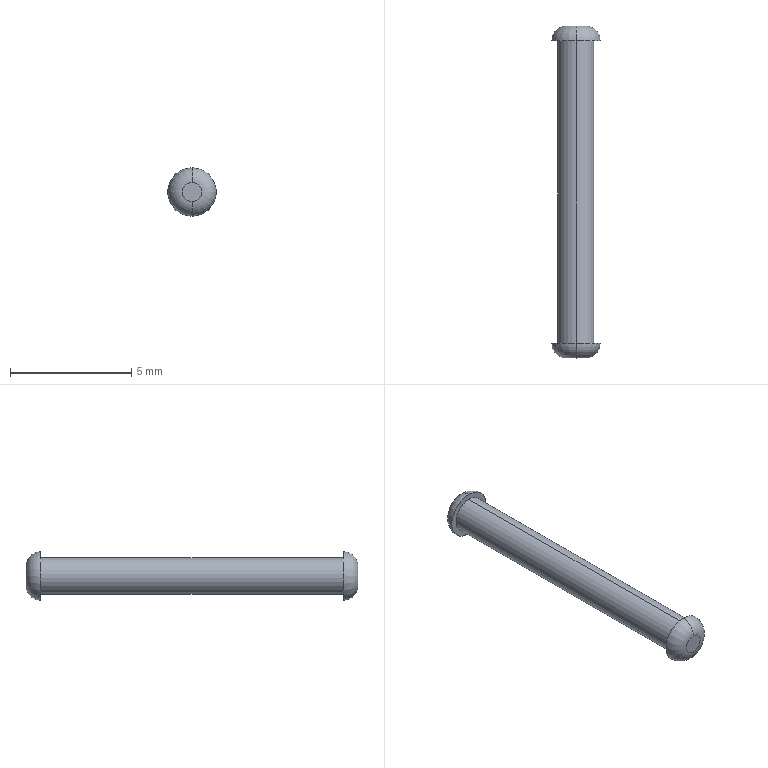Part | SolidWorks | features Extrusion 1, Fillet 1, ICE 1, MirrorPattern 1 | 1 solid | 10 faces | box 2 x 13.7 x 2 mm | volume 25.019 mm3 | torus 4 | plane 4 | cylinder 2 | commonest cylinder face diameters 1.5 x2
STEP:
#1=CARTESIAN_POINT('',(0.,-6.25,1.));
#2=VERTEX_POINT('',#1);
#3=CARTESIAN_POINT('',(0.,-6.25,-1.));
#4=VERTEX_POINT('',#3);
#5=CARTESIAN_POINT('',(0.,-6.25,0.));
#6=DIRECTION('',(0.,1.,0.));
#7=DIRECTION('',(0.,0.,1.));
#8=AXIS2_PLACEMENT_3D('',#5,#6,#7);
#9=CIRCLE('',#8,1.);
#10=EDGE_CURVE('',#2,#4,#9,.T.);
#11=ORIENTED_EDGE('',*,*,#10,.F.);
#12=CARTESIAN_POINT('',(0.,-6.85,0.4));
#13=VERTEX_POINT('',#12);
#14=CARTESIAN_POINT('',(0.,-6.25,0.4));
#15=DIRECTION('',(1.,0.,0.));
#16=DIRECTION('',(0.,0.,-1.));
#17=AXIS2_PLACEMENT_3D('',#14,#15,#16);
#18=CIRCLE('',#17,0.6);
#19=EDGE_CURVE('',#2,#13,#18,.T.);
#20=ORIENTED_EDGE('',*,*,#19,.T.);
#21=CARTESIAN_POINT('',(0.,-6.85,-0.4));
#22=VERTEX_POINT('',#21);
#23=CARTESIAN_POINT('',(0.,-6.85,0.));
#24=DIRECTION('',(0.,-1.,0.));
#25=DIRECTION('',(0.,0.,-1.));
#26=AXIS2_PLACEMENT_3D('',#23,#24,#25);
#27=CIRCLE('',#26,0.4);
#28=EDGE_CURVE('',#22,#13,#27,.T.);
#29=ORIENTED_EDGE('',*,*,#28,.F.);
#30=CARTESIAN_POINT('',(0.,-6.25,-0.4));
#31=DIRECTION('',(-1.,0.,0.));
#32=DIRECTION('',(0.,0.,1.));
#33=AXIS2_PLACEMENT_3D('',#30,#31,#32);
#34=CIRCLE('',#33,0.6);
#35=EDGE_CURVE('',#4,#22,#34,.T.);
#36=ORIENTED_EDGE('',*,*,#35,.F.);
#37=EDGE_LOOP('',(#11,#20,#29,#36));
#38=FACE_OUTER_BOUND('',#37,.T.);
#39=CARTESIAN_POINT('',(0.,-6.25,0.));
#40=DIRECTION('',(0.,-1.,0.));
#41=DIRECTION('',(0.,0.,-1.));
#42=AXIS2_PLACEMENT_3D('',#39,#40,#41);
#43=TOROIDAL_SURFACE('',#42,0.4,0.6);
#44=ADVANCED_FACE('',(#38),#43,.T.);
#45=CARTESIAN_POINT('',(0.,6.25,1.));
#46=VERTEX_POINT('',#45);
#47=CARTESIAN_POINT('',(0.,6.25,-1.));
#48=VERTEX_POINT('',#47);
#49=CARTESIAN_POINT('',(0.,6.25,0.));
#50=DIRECTION('',(0.,1.,0.));
#51=DIRECTION('',(0.,0.,1.));
#52=AXIS2_PLACEMENT_3D('',#49,#50,#51);
#53=CIRCLE('',#52,1.);
#54=EDGE_CURVE('',#46,#48,#53,.T.);
#55=ORIENTED_EDGE('',*,*,#54,.T.);
#56=CARTESIAN_POINT('',(0.,6.85,-0.4));
#57=VERTEX_POINT('',#56);
#58=CARTESIAN_POINT('',(0.,6.25,-0.4));
#59=DIRECTION('',(1.,0.,0.));
#60=DIRECTION('',(0.,0.,-1.));
#61=AXIS2_PLACEMENT_3D('',#58,#59,#60);
#62=CIRCLE('',#61,0.6);
#63=EDGE_CURVE('',#48,#57,#62,.T.);
#64=ORIENTED_EDGE('',*,*,#63,.T.);
#65=CARTESIAN_POINT('',(0.,6.85,0.4));
#66=VERTEX_POINT('',#65);
#67=CARTESIAN_POINT('',(0.,6.85,0.));
#68=DIRECTION('',(0.,1.,0.));
#69=DIRECTION('',(0.,0.,1.));
#70=AXIS2_PLACEMENT_3D('',#67,#68,#69);
#71=CIRCLE('',#70,0.4);
#72=EDGE_CURVE('',#66,#57,#71,.T.);
#73=ORIENTED_EDGE('',*,*,#72,.F.);
#74=CARTESIAN_POINT('',(0.,6.25,0.4));
#75=DIRECTION('',(-1.,0.,0.));
#76=DIRECTION('',(0.,0.,1.));
#77=AXIS2_PLACEMENT_3D('',#74,#75,#76);
#78=CIRCLE('',#77,0.6);
#79=EDGE_CURVE('',#46,#66,#78,.T.);
#80=ORIENTED_EDGE('',*,*,#79,.F.);
#81=EDGE_LOOP('',(#55,#64,#73,#80));
#82=FACE_OUTER_BOUND('',#81,.T.);
#83=CARTESIAN_POINT('',(0.,6.25,0.));
#84=DIRECTION('',(0.,1.,0.));
#85=DIRECTION('',(0.,0.,1.));
#86=AXIS2_PLACEMENT_3D('',#83,#84,#85);
#87=TOROIDAL_SURFACE('',#86,0.4,0.6);
#88=ADVANCED_FACE('',(#82),#87,.T.);
#89=CARTESIAN_POINT('',(0.,6.25,0.75));
#90=VERTEX_POINT('',#89);
#91=CARTESIAN_POINT('',(0.,6.25,-0.75));
#92=VERTEX_POINT('',#91);
#93=CARTESIAN_POINT('',(0.,6.25,0.));
#94=DIRECTION('',(0.,1.,0.));
#95=DIRECTION('',(0.,0.,1.));
#96=AXIS2_PLACEMENT_3D('',#93,#94,#95);
#97=CIRCLE('',#96,0.75);
#98=EDGE_CURVE('',#90,#92,#97,.T.);
#99=ORIENTED_EDGE('',*,*,#98,.F.);
#100=CARTESIAN_POINT('',(0.,-6.25,0.75));
#101=VERTEX_POINT('',#100);
#102=CARTESIAN_POINT('',(0.,6.25,0.75));
#103=DIRECTION('',(0.,-1.,0.));
#104=VECTOR('',#103,1000.);
#105=LINE('',#102,#104);
#106=EDGE_CURVE('',#90,#101,#105,.T.);
#107=ORIENTED_EDGE('',*,*,#106,.T.);
#108=CARTESIAN_POINT('',(0.,-6.25,-0.75));
#109=VERTEX_POINT('',#108);
#110=CARTESIAN_POINT('',(0.,-6.25,0.));
#111=DIRECTION('',(0.,1.,0.));
#112=DIRECTION('',(0.,0.,1.));
#113=AXIS2_PLACEMENT_3D('',#110,#111,#112);
#114=CIRCLE('',#113,0.75);
#115=EDGE_CURVE('',#101,#109,#114,.T.);
#116=ORIENTED_EDGE('',*,*,#115,.T.);
#117=CARTESIAN_POINT('',(0.,6.25,-0.75));
#118=DIRECTION('',(0.,-1.,0.));
#119=VECTOR('',#118,1000.);
#120=LINE('',#117,#119);
#121=EDGE_CURVE('',#92,#109,#120,.T.);
#122=ORIENTED_EDGE('',*,*,#121,.F.);
#123=EDGE_LOOP('',(#99,#107,#116,#122));
#124=FACE_OUTER_BOUND('',#123,.T.);
#125=CARTESIAN_POINT('',(0.,6.25,0.));
#126=DIRECTION('',(0.,-1.,0.));
#127=DIRECTION('',(0.,0.,-1.));
#128=AXIS2_PLACEMENT_3D('',#125,#126,#127);
#129=CYLINDRICAL_SURFACE('',#128,0.75);
#130=ADVANCED_FACE('',(#124),#129,.T.);
#131=ORIENTED_EDGE('',*,*,#106,.F.);
#132=CARTESIAN_POINT('',(0.,6.25,0.));
#133=DIRECTION('',(0.,1.,0.));
#134=DIRECTION('',(0.,0.,1.));
#135=AXIS2_PLACEMENT_3D('',#132,#133,#134);
#136=CIRCLE('',#135,0.75);
#137=EDGE_CURVE('',#92,#90,#136,.T.);
#138=ORIENTED_EDGE('',*,*,#137,.F.);
#139=ORIENTED_EDGE('',*,*,#121,.T.);
#140=CARTESIAN_POINT('',(0.,-6.25,0.));
#141=DIRECTION('',(0.,1.,0.));
#142=DIRECTION('',(0.,0.,1.));
#143=AXIS2_PLACEMENT_3D('',#140,#141,#142);
#144=CIRCLE('',#143,0.75);
#145=EDGE_CURVE('',#109,#101,#144,.T.);
#146=ORIENTED_EDGE('',*,*,#145,.T.);
#147=EDGE_LOOP('',(#131,#138,#139,#146));
#148=FACE_OUTER_BOUND('',#147,.T.);
#149=CARTESIAN_POINT('',(0.,6.25,0.));
#150=DIRECTION('',(0.,-1.,0.));
#151=DIRECTION('',(0.,0.,-1.));
#152=AXIS2_PLACEMENT_3D('',#149,#150,#151);
#153=CYLINDRICAL_SURFACE('',#152,0.75);
#154=ADVANCED_FACE('',(#148),#153,.T.);
#155=ORIENTED_EDGE('',*,*,#72,.T.);
#156=CARTESIAN_POINT('',(0.,6.85,0.));
#157=DIRECTION('',(0.,1.,0.));
#158=DIRECTION('',(0.,0.,1.));
#159=AXIS2_PLACEMENT_3D('',#156,#157,#158);
#160=CIRCLE('',#159,0.4);
#161=EDGE_CURVE('',#57,#66,#160,.T.);
#162=ORIENTED_EDGE('',*,*,#161,.T.);
#163=EDGE_LOOP('',(#155,#162));
#164=FACE_OUTER_BOUND('',#163,.T.);
#165=CARTESIAN_POINT('',(0.,6.85,0.));
#166=DIRECTION('',(0.,1.,0.));
#167=DIRECTION('',(0.,0.,1.));
#168=AXIS2_PLACEMENT_3D('',#165,#166,#167);
#169=PLANE('',#168);
#170=ADVANCED_FACE('',(#164),#169,.T.);
#171=ORIENTED_EDGE('',*,*,#137,.T.);
#172=ORIENTED_EDGE('',*,*,#98,.T.);
#173=EDGE_LOOP('',(#171,#172));
#174=FACE_BOUND('',#173,.T.);
#175=ORIENTED_EDGE('',*,*,#54,.F.);
#176=CARTESIAN_POINT('',(0.,6.25,0.));
#177=DIRECTION('',(0.,1.,0.));
#178=DIRECTION('',(0.,0.,1.));
#179=AXIS2_PLACEMENT_3D('',#176,#177,#178);
#180=CIRCLE('',#179,1.);
#181=EDGE_CURVE('',#48,#46,#180,.T.);
#182=ORIENTED_EDGE('',*,*,#181,.F.);
#183=EDGE_LOOP('',(#175,#182));
#184=FACE_OUTER_BOUND('',#183,.T.);
#185=CARTESIAN_POINT('',(0.,6.25,0.));
#186=DIRECTION('',(0.,1.,0.));
#187=DIRECTION('',(0.,0.,1.));
#188=AXIS2_PLACEMENT_3D('',#185,#186,#187);
#189=PLANE('',#188);
#190=ADVANCED_FACE('',(#174,#184),#189,.F.);
#191=ORIENTED_EDGE('',*,*,#63,.F.);
#192=ORIENTED_EDGE('',*,*,#181,.T.);
#193=ORIENTED_EDGE('',*,*,#79,.T.);
#194=ORIENTED_EDGE('',*,*,#161,.F.);
#195=EDGE_LOOP('',(#191,#192,#193,#194));
#196=FACE_OUTER_BOUND('',#195,.T.);
#197=CARTESIAN_POINT('',(0.,6.25,0.));
#198=DIRECTION('',(0.,1.,0.));
#199=DIRECTION('',(0.,0.,1.));
#200=AXIS2_PLACEMENT_3D('',#197,#198,#199);
#201=TOROIDAL_SURFACE('',#200,0.4,0.6);
#202=ADVANCED_FACE('',(#196),#201,.T.);
#203=ORIENTED_EDGE('',*,*,#28,.T.);
#204=CARTESIAN_POINT('',(0.,-6.85,0.));
#205=DIRECTION('',(0.,-1.,0.));
#206=DIRECTION('',(0.,0.,-1.));
#207=AXIS2_PLACEMENT_3D('',#204,#205,#206);
#208=CIRCLE('',#207,0.4);
#209=EDGE_CURVE('',#13,#22,#208,.T.);
#210=ORIENTED_EDGE('',*,*,#209,.T.);
#211=EDGE_LOOP('',(#203,#210));
#212=FACE_OUTER_BOUND('',#211,.T.);
#213=CARTESIAN_POINT('',(0.,-6.85,0.));
#214=DIRECTION('',(0.,-1.,0.));
#215=DIRECTION('',(0.,0.,1.));
#216=AXIS2_PLACEMENT_3D('',#213,#214,#215);
#217=PLANE('',#216);
#218=ADVANCED_FACE('',(#212),#217,.T.);
#219=ORIENTED_EDGE('',*,*,#145,.F.);
#220=ORIENTED_EDGE('',*,*,#115,.F.);
#221=EDGE_LOOP('',(#219,#220));
#222=FACE_BOUND('',#221,.T.);
#223=CARTESIAN_POINT('',(0.,-6.25,0.));
#224=DIRECTION('',(0.,1.,0.));
#225=DIRECTION('',(0.,0.,1.));
#226=AXIS2_PLACEMENT_3D('',#223,#224,#225);
#227=CIRCLE('',#226,1.);
#228=EDGE_CURVE('',#4,#2,#227,.T.);
#229=ORIENTED_EDGE('',*,*,#228,.T.);
#230=ORIENTED_EDGE('',*,*,#10,.T.);
#231=EDGE_LOOP('',(#229,#230));
#232=FACE_OUTER_BOUND('',#231,.T.);
#233=CARTESIAN_POINT('',(0.,-6.25,0.));
#234=DIRECTION('',(0.,-1.,0.));
#235=DIRECTION('',(0.,0.,1.));
#236=AXIS2_PLACEMENT_3D('',#233,#234,#235);
#237=PLANE('',#236);
#238=ADVANCED_FACE('',(#222,#232),#237,.F.);
#239=ORIENTED_EDGE('',*,*,#19,.F.);
#240=ORIENTED_EDGE('',*,*,#228,.F.);
#241=ORIENTED_EDGE('',*,*,#35,.T.);
#242=ORIENTED_EDGE('',*,*,#209,.F.);
#243=EDGE_LOOP('',(#239,#240,#241,#242));
#244=FACE_OUTER_BOUND('',#243,.T.);
#245=CARTESIAN_POINT('',(0.,-6.25,0.));
#246=DIRECTION('',(0.,-1.,0.));
#247=DIRECTION('',(0.,0.,-1.));
#248=AXIS2_PLACEMENT_3D('',#245,#246,#247);
#249=TOROIDAL_SURFACE('',#248,0.4,0.6);
#250=ADVANCED_FACE('',(#244),#249,.T.);
#251=CLOSED_SHELL('',(#44,#88,#130,#154,#170,#190,#202,#218,#238,#250));
#252=MANIFOLD_SOLID_BREP('',#251);
#253=CARTESIAN_POINT('',(0.,0.,0.));
#254=DIRECTION('',(0.,0.,1.));
#255=DIRECTION('',(1.,0.,0.));
#256=AXIS2_PLACEMENT_3D('',#253,#254,#255);
#257=(LENGTH_UNIT()NAMED_UNIT(*)SI_UNIT(.MILLI.,.METRE.));
#258=UNCERTAINTY_MEASURE_WITH_UNIT(LENGTH_MEASURE(0.00001),#257,'','');
#259=(NAMED_UNIT(*)PLANE_ANGLE_UNIT()SI_UNIT($,.RADIAN.));
#260=(NAMED_UNIT(*)SI_UNIT($,.STERADIAN.)SOLID_ANGLE_UNIT());
#261=(GEOMETRIC_REPRESENTATION_CONTEXT(3)GLOBAL_UNCERTAINTY_ASSIGNED_CONTEXT((#258))GLOBAL_UNIT_ASSIGNED_CONTEXT((#257,#259,#260))REPRESENTATION_CONTEXT('',''));
#262=ADVANCED_BREP_SHAPE_REPRESENTATION('',(#252,#256),#261);